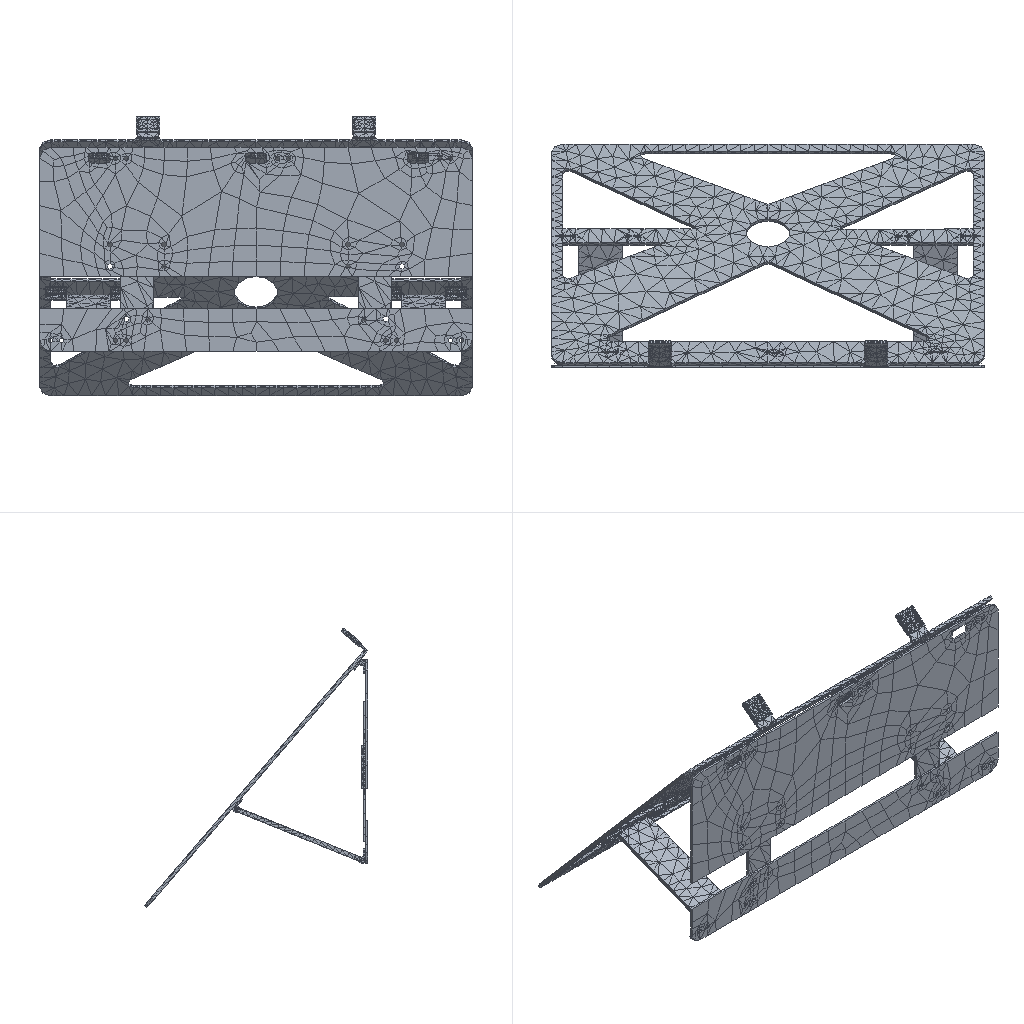Simulation study | ansys workbench
Set-up summary:
category,name,step,type,value,unit,region
solver,ansys_workbench
units,mm-N-s-tonne (MPa),,stated,"/units,MPA"
analysis,LS1,,static
load_step,LS1,LS1,static,nsubst=1; time=1
mesh,nodes,,,34982
mesh,elements,,,26385
element_type,SOLID187,,,13031
element_type,TARGE170,,,5865
element_type,CONTA174,,,5865
element_type,SURF154,,,992
element_type,SOLID186,,,632
material,Structural Steel,,E,200000,tonne s^-2 mm^-1
material,Structural Steel,,nu,0.3
material,Structural Steel,,density,7.85e-09,tonne mm^-3
material,Structural Steel,,conductivity,60.5,tonne mm s^-3 C^-1
material,Structural Steel,,specific_heat,4.34e+08,mm^2 s^-2 C^-1
material,Structural Steel,,cte,1.2e-05,C^-1
material,Structural Steel,,permeability,10000
material,Structural Steel,,resistivity,0.00017,ohm mm
load,Define Force Using Surface Effect Elements,LS1,surface-effect pres face 1,-1.28788e-17,,SURF154 #153
load,Define Force Using Surface Effect Elements,LS1,surface-effect pres face 2,-0.004879,,SURF154 #153
load,Define Force Using Surface Effect Elements,LS1,surface-effect pres face 3,-0.004202,,SURF154 #153
bc,Fixed Supports,model,fixed,[dofs=ALL],,_FIXEDSU
contact,Contact Region,,bonded (always),element=CONTA174
contact,Contact Region 2,,bonded (always),element=CONTA174
contact,Contact Region 3,,bonded (always),element=CONTA174
contact,Contact Region 4,,bonded (always),element=CONTA174
contact,Contact Region 5,,bonded (always),element=CONTA174
contact,Contact Region 6,,bonded (always),element=CONTA174
contact,Contact Region 7,,bonded (always),element=CONTA174
contact,Contact Region 8,,bonded (always),element=CONTA174
contact,Contact Region 9,,bonded (always),element=CONTA174
contact,Contact Region 10,,bonded (always),element=CONTA174
contact,Contact Region 11,,bonded (always),element=CONTA174
contact,Contact Region 12,,bonded (always),element=CONTA174
contact,Contact Region 13,,bonded (always),element=CONTA174
contact,Contact Region 14,,bonded (always),element=CONTA174
contact,Contact Region 15,,bonded (always),element=CONTA174
contact,Contact Region 16,,bonded (always),element=CONTA174
contact,Contact Region 17,,bonded (always),element=CONTA174
contact,Contact Region 18,,bonded (always),element=CONTA174
contact,Contact Region 19,,bonded (always),element=CONTA174
contact,Contact Region 20,,bonded (always),element=CONTA174
contact,Contact Region 21,,bonded (always),element=CONTA174
contact,Contact Region 22,,bonded (always),element=CONTA174
contact,Contact Region 23,,bonded (always),element=CONTA174
contact,Contact Region 24,,bonded (always),element=CONTA174
contact,Contact Region 25,,bonded (always),element=CONTA174
contact,Contact Region 26,,bonded (always),element=CONTA174
contact,Contact Region 27,,bonded (always),element=CONTA174
contact,Contact Region 28,,bonded (always),element=CONTA174
contact,Contact Region 29,,bonded (always),element=CONTA174
contact,Contact Region 30,,bonded (always),element=CONTA174
contact,Contact Region 31,,bonded (always),element=CONTA174
contact,Contact Region 32,,bonded (always),element=CONTA174
contact,Contact Region 33,,bonded (always),element=CONTA174
contact,Contact Region 34,,bonded (always),element=CONTA174
contact,Contact Region 35,,bonded (always),element=CONTA174
contact,Contact Region 36,,bonded (always),element=CONTA174
contact,Contact Region 37,,bonded (always),element=CONTA174
contact,Contact Region 38,,bonded (always),element=CONTA174
contact,Contact Region 39,,bonded (always),element=CONTA174
contact,Contact Region 40,,bonded (always),element=CONTA174
contact,Contact Region 41,,bonded (always),element=CONTA174
contact,Contact Region 42,,bonded (always),element=CONTA174
contact,Contact Region 43,,bonded (always),element=CONTA174
contact,Contact Region 44,,bonded (always),element=CONTA174
contact,Contact Region 45,,bonded (always),element=CONTA174
contact,Contact Region 46,,bonded (always),element=CONTA174
contact,Contact Region 47,,bonded (always),element=CONTA174
contact,Contact Region 48,,bonded (always),element=CONTA174
contact,Contact Region 49,,bonded (always),element=CONTA174
contact,Contact Region 50,,bonded (always),element=CONTA174
contact,Contact Region 51,,bonded (always),element=CONTA174
contact,Contact Region 52,,bonded (always),element=CONTA174
contact,Contact Region 53,,bonded (always),element=CONTA174
contact,Contact Region 54,,bonded (always),element=CONTA174
contact,Contact Region 55,,bonded (always),element=CONTA174
contact,Contact Region 56,,bonded (always),element=CONTA174
contact,Contact Region 57,,bonded (always),element=CONTA174
contact,Contact Region 58,,bonded (always),element=CONTA174
contact,Contact Region 59,,bonded (always),element=CONTA174
contact,Contact Region 60,,bonded (always),element=CONTA174
contact,Contact Region 61,,bonded (always),element=CONTA174
named_set,_FIXEDSU,,node,1923
Ansys APDL input file, long lists of numbers shortened:
/batch
/config,noeldb,1     ! force off writing results to database
*get,_wallstrt,active,,time,wall
! ANSYS input file written by Workbench version 2022 R1
! File used for geometry attach:
/title,wbnew--____ (A5)
! ****** Begin Custom Load Command Snippet ******
/COM, ACT Extensions:
/COM,     LSDYNA, 2021.1
/COM,
! ****** End   Custom Load Command Snippet ******
*DIM,_wb_ProjectScratch_dir,string,248
_wb_ProjectScratch_dir(1) = ''
*DIM,_wb_SolverFiles_dir,string,248
_wb_SolverFiles_dir(1) = ''
*DIM,_wb_userfiles_dir,string,248
_wb_userfiles_dir(1) = ''
/com,--- Data in consistent NMM units. See Solving Units in the help system for more information.
/units,MPA
/nopr
/wb,file,start              !  signify a WB generated input file
/prep7
! Turn off shape checking because checks already performed inside WB mesher.
! See help system for more information.
SHPP,OFF,,NOWARN
/nolist
etcon,set             ! allow ANSYS to choose best KEYOP's for 180x elements, resets any applicable keyopt to MAPDL defaults
/com,*********** Nodes for the whole assembly ***********
nblock,3,,38480
(1i9,3e20.9e3)
        1     3.182810886E+02     2.161891006E+02     1.535110388E+02
! (34981 more lines like these left out)
-1
/wb,elem,start            !  set before creation of elements
/com,*********** Elements for Body 1 "fromt_backplate_with_mount_assy___ _________|front-backplate___ _________|__________2" ***********
et,1,186
keyo,1,2,1          ! set full integration on SOLID186
eblock,19,solid,,359
(19i9)
        1        1        1        1        0        0        0        0       20        0    13305    32083    32585    32584    32687    32522    32888    32889    32789
! (717 more lines like these left out)
-1
/com,*********** Elements for Body 2 "fromt_backplate_with_mount_assy___ _________|sliding_system_mount___ _________|_______-________2" ***********
et,2,187
eblock,19,solid,,223
(19i9)
        2        2        2        2        0        0        0        0       10        0     1339     3144     3192     3145     3200     3429     3434     3426     3430
! (445 more lines like these left out)
-1
/com,*********** Elements for Body 3 "fromt_backplate_with_mount_assy___ _________|sliding_system_mount___ _________|_______-________2[2]" ***********
et,3,187
eblock,19,solid,,223
(19i9)
        3        3        3        3        0        0        0        0       10        0    11173    26097    26145    26098    26153    26382    26387    26379    26383
! (445 more lines like these left out)
-1
/com,*********** Elements for Body 4 "fromt_backplate_with_mount_assy___ _________|sliding_system_mount___ _________|_______-________2[3]" ***********
et,4,187
eblock,19,solid,,223
(19i9)
        4        4        4        4        0        0        0        0       10        0     1562     3692     3740     3693     3748     3977     3982     3974     3978
! (445 more lines like these left out)
-1
/com,*********** Elements for Body 5 "fromt_backplate_with_mount_assy___ _________|sliding_system_mount___ _________|_______-________2[4]" ***********
et,5,187
eblock,19,solid,,223
(19i9)
        5        5        5        5        0        0        0        0       10        0     2179     5406     5454     5407     5462     5691     5696     5688     5692
! (445 more lines like these left out)
-1
! (25 more sections like these left out)
/wb,elem,end               !  done creating elements
/com,*********** Send User Defined Coordinate System(s) ***********
csys,0
toffst,273.15,  ! Temperature offset from absolute zero
/com,*********** Set Reference Temperature ***********
tref,22.
/wb,mat,start              !  starting to send materials
/com,*********** Send Materials ***********
Temperature = 'TEMP' ! Temperature
MP,DENS,1,7.85e-09,	! tonne mm^-3
MP,ALPX,1,1.2e-05,	! C^-1
MP,C,1,434000000,	! mm^2 s^-2 C^-1
MP,KXX,1,60.5,	! tonne mm s^-3 C^-1
MP,RSVX,1,0.00017,	! ohm mm
MP,EX,1,200000,	! tonne s^-2 mm^-1
MP,NUXY,1,0.3,
MP,MURX,1,10000,
Temperature = 'TEMP' ! Temperature
MP,DENS,2,7.85e-09,	! tonne mm^-3
MP,ALPX,2,1.2e-05,	! C^-1
MP,C,2,434000000,	! mm^2 s^-2 C^-1
MP,KXX,2,60.5,	! tonne mm s^-3 C^-1
MP,RSVX,2,0.00017,	! ohm mm
MP,EX,2,200000,	! tonne s^-2 mm^-1
MP,NUXY,2,0.3,
MP,MURX,2,10000,
Temperature = 'TEMP' ! Temperature
MP,DENS,3,7.85e-09,	! tonne mm^-3
MP,ALPX,3,1.2e-05,	! C^-1
MP,C,3,434000000,	! mm^2 s^-2 C^-1
MP,KXX,3,60.5,	! tonne mm s^-3 C^-1
MP,RSVX,3,0.00017,	! ohm mm
MP,EX,3,200000,	! tonne s^-2 mm^-1
MP,NUXY,3,0.3,
MP,MURX,3,10000,
Temperature = 'TEMP' ! Temperature
MP,DENS,4,7.85e-09,	! tonne mm^-3
MP,ALPX,4,1.2e-05,	! C^-1
MP,C,4,434000000,	! mm^2 s^-2 C^-1
MP,KXX,4,60.5,	! tonne mm s^-3 C^-1
MP,RSVX,4,0.00017,	! ohm mm
MP,EX,4,200000,	! tonne s^-2 mm^-1
MP,NUXY,4,0.3,
MP,MURX,4,10000,
Temperature = 'TEMP' ! Temperature
MP,DENS,5,7.85e-09,	! tonne mm^-3
MP,ALPX,5,1.2e-05,	! C^-1
MP,C,5,434000000,	! mm^2 s^-2 C^-1
MP,KXX,5,60.5,	! tonne mm s^-3 C^-1
MP,RSVX,5,0.00017,	! ohm mm
MP,EX,5,200000,	! tonne s^-2 mm^-1
MP,NUXY,5,0.3,
MP,MURX,5,10000,
Temperature = 'TEMP' ! Temperature
MP,DENS,6,7.85e-09,	! tonne mm^-3
MP,ALPX,6,1.2e-05,	! C^-1
MP,C,6,434000000,	! mm^2 s^-2 C^-1
MP,KXX,6,60.5,	! tonne mm s^-3 C^-1
MP,RSVX,6,0.00017,	! ohm mm
MP,EX,6,200000,	! tonne s^-2 mm^-1
MP,NUXY,6,0.3,
MP,MURX,6,10000,
Temperature = 'TEMP' ! Temperature
MP,DENS,7,7.85e-09,	! tonne mm^-3
MP,ALPX,7,1.2e-05,	! C^-1
MP,C,7,434000000,	! mm^2 s^-2 C^-1
MP,KXX,7,60.5,	! tonne mm s^-3 C^-1
MP,RSVX,7,0.00017,	! ohm mm
MP,EX,7,200000,	! tonne s^-2 mm^-1
MP,NUXY,7,0.3,
MP,MURX,7,10000,
Temperature = 'TEMP' ! Temperature
MP,DENS,8,7.85e-09,	! tonne mm^-3
MP,ALPX,8,1.2e-05,	! C^-1
MP,C,8,434000000,	! mm^2 s^-2 C^-1
MP,KXX,8,60.5,	! tonne mm s^-3 C^-1
MP,RSVX,8,0.00017,	! ohm mm
MP,EX,8,200000,	! tonne s^-2 mm^-1
MP,NUXY,8,0.3,
MP,MURX,8,10000,
Temperature = 'TEMP' ! Temperature
MP,DENS,9,7.85e-09,	! tonne mm^-3
MP,ALPX,9,1.2e-05,	! C^-1
MP,C,9,434000000,	! mm^2 s^-2 C^-1
MP,KXX,9,60.5,	! tonne mm s^-3 C^-1
MP,RSVX,9,0.00017,	! ohm mm
MP,EX,9,200000,	! tonne s^-2 mm^-1
! (191 more lines like these left out)
/wb,mat,end                !  done sending materials
!************************* Model Summary ********************
!fromt_backplate_with_mount_assy___ _________|front-backplate___ _________|__________2,	结构钢,	matid,	1
!fromt_backplate_with_mount_assy___ _________|sliding_system_mount___ _________|_______-________2,	结构钢,	matid,	2
!fromt_backplate_with_mount_assy___ _________|sliding_system_mount___ _________|_______-________2[2],	结构钢,	matid,	3
! (29 more lines like these left out)
*get,_xmin,node,,mnloc,x
*get,_ymin,node,,mnloc,y
*get,_zmin,node,,mnloc,z
*get,_xmax,node,,mxloc,x
*get,_ymax,node,,mxloc,y
*get,_zmax,node,,mxloc,z
_ASMDIAG=(_xmax-_xmin)*(_xmax-_xmin)+(_ymax-_ymin)*(_ymax-_ymin)+(_zmax-_zmin)*(_zmax-_zmin)
_ASMDIAG=SQRT(_ASMDIAG)
/wb,contact,start          !  starting to send contact
/com,*********** Create Contact "接触区域" ***********
/com,            Real Constant Set For Above Contact Is 32 & 31
*set,tid,32
*set,cid,31
r,tid
r,cid
et,tid,170
et,cid,174
eblock,10,,,30
(15i9)
    26408       32       32       32        0    32628    32629    32088    32302    34569    33086    33083    33780
! (29 more lines like these left out)
-1
eblock,10,,,30
(15i9)
    26438       31       31       31        0    32628    32629    32088    32302    34569    33086    33083    33780
! (29 more lines like these left out)
-1
eblock,10,,,40
(15i9)
    26468       31       32       31        0     3152     3157     3158     3158     3459     3480     3158     3460
! (39 more lines like these left out)
-1
eblock,10,,,40
(15i9)
    26508       32       31       32        0     3152     3157     3158     3158     3459     3480     3158     3460
! (39 more lines like these left out)
-1
keyo,cid,8,2               ! auto create asymmetric contact (from Program Controlled setting)
keyo,cid,10,0              ! adjust contact stiffness each NR iteration (from Program Controlled setting)
keyo,cid,12,5              ! bonded always
keyo,cid,18,1              ! small sliding turned on by application
keyo,cid,2,0               ! augmented Lagrange (from Program Controlled setting)
keyo,cid,4,0               ! on Gauss point (from Program Controlled setting)
keyo,cid,9,1               ! ignore initial gaps/penetration
keyo,cid,7,0               ! No Prediction
rmod,tid,3,10.      ! FKN
rmod,tid,5,0.       ! ICONT
rmod,tid,6,0.       ! PINB
rmod,tid,10,0.      ! CNOF
rmod,tid,12,0.      ! FKT
rmod,tid,36,113     ! WB DSID
rmod,cid,3,10.      ! FKN
rmod,cid,5,0.       ! ICONT
rmod,cid,6,0.       ! PINB
rmod,cid,10,0.      ! CNOF
rmod,cid,12,0.      ! FKT
rmod,cid,36,113     ! WB DSID
/com,*********** Create Contact "接触区域 2" ***********
/com,            Real Constant Set For Above Contact Is 34 & 33
*set,tid,34
*set,cid,33
r,tid
r,cid
et,tid,170
et,cid,174
eblock,10,,,30
(15i9)
    26548       34       34       34        0    32142    32258    32259    32293    33301    33692    33696    33302
! (29 more lines like these left out)
-1
eblock,10,,,30
(15i9)
    26578       33       33       33        0    32142    32258    32259    32293    33301    33692    33696    33302
! (29 more lines like these left out)
-1
eblock,10,,,40
(15i9)
    26608       33       34       33        0    26105    26110    26111    26111    26412    26433    26111    26413
! (39 more lines like these left out)
-1
eblock,10,,,40
(15i9)
    26648       34       33       34        0    26105    26110    26111    26111    26412    26433    26111    26413
! (39 more lines like these left out)
-1
keyo,cid,8,2               ! auto create asymmetric contact (from Program Controlled setting)
keyo,cid,10,0              ! adjust contact stiffness each NR iteration (from Program Controlled setting)
keyo,cid,12,5              ! bonded always
keyo,cid,18,1              ! small sliding turned on by application
keyo,cid,2,0               ! augmented Lagrange (from Program Controlled setting)
keyo,cid,4,0               ! on Gauss point (from Program Controlled setting)
keyo,cid,9,1               ! ignore initial gaps/penetration
keyo,cid,7,0               ! No Prediction
rmod,tid,3,10.      ! FKN
rmod,tid,5,0.       ! ICONT
rmod,tid,6,0.       ! PINB
rmod,tid,10,0.      ! CNOF
rmod,tid,12,0.      ! FKT
rmod,tid,36,116     ! WB DSID
rmod,cid,3,10.      ! FKN
rmod,cid,5,0.       ! ICONT
rmod,cid,6,0.       ! PINB
rmod,cid,10,0.      ! CNOF
rmod,cid,12,0.      ! FKT
rmod,cid,36,116     ! WB DSID
/com,*********** Create Contact "接触区域 3" ***********
/com,            Real Constant Set For Above Contact Is 36 & 35
*set,tid,36
*set,cid,35
r,tid
r,cid
et,tid,170
et,cid,174
eblock,10,,,28
(15i9)
    26688       36       36       36        0    32119    32092    32138    32091    33104    33105    33098    33097
! (27 more lines like these left out)
-1
eblock,10,,,28
(15i9)
    26716       35       35       35        0    32119    32092    32138    32091    33104    33105    33098    33097
! (27 more lines like these left out)
-1
eblock,10,,,40
(15i9)
    26744       35       36       35        0     3700     3705     3706     3706     4007     4028     3706     4008
! (39 more lines like these left out)
-1
eblock,10,,,40
(15i9)
    26784       36       35       36        0     3700     3705     3706     3706     4007     4028     3706     4008
! (39 more lines like these left out)
-1
keyo,cid,8,2               ! auto create asymmetric contact (from Program Controlled setting)
keyo,cid,10,0              ! adjust contact stiffness each NR iteration (from Program Controlled setting)
keyo,cid,12,5              ! bonded always
keyo,cid,18,1              ! small sliding turned on by application
keyo,cid,2,0               ! augmented Lagrange (from Program Controlled setting)
keyo,cid,4,0               ! on Gauss point (from Program Controlled setting)
keyo,cid,9,1               ! ignore initial gaps/penetration
keyo,cid,7,0               ! No Prediction
rmod,tid,3,10.      ! FKN
rmod,tid,5,0.       ! ICONT
rmod,tid,6,0.       ! PINB
rmod,tid,10,0.      ! CNOF
rmod,tid,12,0.      ! FKT
rmod,tid,36,119     ! WB DSID
rmod,cid,3,10.      ! FKN
rmod,cid,5,0.       ! ICONT
rmod,cid,6,0.       ! PINB
rmod,cid,10,0.      ! CNOF
rmod,cid,12,0.      ! FKT
rmod,cid,36,119     ! WB DSID
/com,*********** Create Contact "接触区域 4" ***********
/com,            Real Constant Set For Above Contact Is 38 & 37
*set,tid,38
*set,cid,37
r,tid
r,cid
et,tid,170
et,cid,174
eblock,10,,,29
(15i9)
    26824       38       38       38        0    32119    32092    32138    32091    33104    33105    33098    33097
! (28 more lines like these left out)
-1
eblock,10,,,29
(15i9)
    26853       37       37       37        0    32119    32092    32138    32091    33104    33105    33098    33097
! (28 more lines like these left out)
-1
eblock,10,,,40
(15i9)
    26882       37       38       37        0     5414     5419     5420     5420     5721     5742     5420     5722
! (39 more lines like these left out)
-1
eblock,10,,,40
(15i9)
    26922       38       37       38        0     5414     5419     5420     5420     5721     5742     5420     5722
! (39 more lines like these left out)
-1
keyo,cid,8,2               ! auto create asymmetric contact (from Program Controlled setting)
keyo,cid,10,0              ! adjust contact stiffness each NR iteration (from Program Controlled setting)
keyo,cid,12,5              ! bonded always
keyo,cid,18,1              ! small sliding turned on by application
keyo,cid,2,0               ! augmented Lagrange (from Program Controlled setting)
keyo,cid,4,0               ! on Gauss point (from Program Controlled setting)
keyo,cid,9,1               ! ignore initial gaps/penetration
keyo,cid,7,0               ! No Prediction
rmod,tid,3,10.      ! FKN
rmod,tid,5,0.       ! ICONT
rmod,tid,6,0.       ! PINB
rmod,tid,10,0.      ! CNOF
rmod,tid,12,0.      ! FKT
rmod,tid,36,122     ! WB DSID
rmod,cid,3,10.      ! FKN
rmod,cid,5,0.       ! ICONT
rmod,cid,6,0.       ! PINB
rmod,cid,10,0.      ! CNOF
rmod,cid,12,0.      ! FKT
rmod,cid,36,122     ! WB DSID
/com,*********** Create Contact "接触区域 5" ***********
/com,            Real Constant Set For Above Contact Is 40 & 39
*set,tid,40
*set,cid,39
r,tid
r,cid
et,tid,170
et,cid,174
eblock,10,,,25
(15i9)
    26962       40       40       40        0    32628    32629    32088    32302    34569    33086    33083    33780
! (24 more lines like these left out)
-1
eblock,10,,,25
(15i9)
    26987       39       39       39        0    32628    32629    32088    32302    34569    33086    33083    33780
! (24 more lines like these left out)
-1
eblock,10,,,15
(15i9)
    27012       39       40       39        0     5087     5079     5006     5009     5341     5194     5191     5203
! (14 more lines like these left out)
-1
eblock,10,,,15
(15i9)
    27027       40       39       40        0     5087     5079     5006     5009     5341     5194     5191     5203
! (14 more lines like these left out)
-1
keyo,cid,8,2               ! auto create asymmetric contact (from Program Controlled setting)
keyo,cid,10,0              ! adjust contact stiffness each NR iteration (from Program Controlled setting)
keyo,cid,12,5              ! bonded always
keyo,cid,18,1              ! small sliding turned on by application
keyo,cid,2,0               ! augmented Lagrange (from Program Controlled setting)
keyo,cid,4,0               ! on Gauss point (from Program Controlled setting)
keyo,cid,9,1               ! ignore initial gaps/penetration
keyo,cid,7,0               ! No Prediction
rmod,tid,3,10.      ! FKN
rmod,tid,5,0.       ! ICONT
rmod,tid,6,0.       ! PINB
rmod,tid,10,0.      ! CNOF
rmod,tid,12,0.      ! FKT
rmod,tid,36,125     ! WB DSID
rmod,cid,3,10.      ! FKN
rmod,cid,5,0.       ! ICONT
rmod,cid,6,0.       ! PINB
rmod,cid,10,0.      ! CNOF
rmod,cid,12,0.      ! FKT
rmod,cid,36,125     ! WB DSID
! (56 more sections like these left out)
/wb,contact,end            !  done creating contacts
/golist
/wb,load,start             !  starting to send loads
/com,*********** Fixed Supports ***********
CMBLOCK,_FIXEDSU,NODE,     1923
(8i10)
     30176     30177     30178     30179     30180     30181     30182     30183
! (240 more lines like these left out)
cmsel,s,_FIXEDSU
d,all,all
nsel,all
/com,*********** Define Force Using Surface Effect Elements ***********
local,12,0,0.,0.,0.,0.,0.,0.
csys,0
et,153,154
eblock,10,,,992
(15i9)
    38138      153      153      153       12    11615    12008    11616    11616    14263    14269    11616    14260
! (991 more lines like these left out)
-1
esel,s,type,,153
keyop,153,2,1                ! Apply load in local coordinate system
keyop,153,7,1                ! Use original area so load is constant in large deformation
esel,all
/gst,on,on
fini
*get,_numnode,node,0,count
*get,_numelem,elem,0,count
*get, _MAXELEMNUM, elem, 0, NUM, MAX
*get, _MAXNODENUM, node, 0, NUM, MAX
*get, _MAXELEMTYPE, etyp, 0, NUM, MAX
*get, _MAXREALCONST, real, 0, NUM, MAX
/go
/wb,load,end               !  done creating loads
/com,--- Number of total nodes = %_numnode%
/com,--- Number of contact elements = 12722
/com,--- Number of spring elements = 0
/com,--- Number of bearing elements = 0
/com,--- Number of solid elements = 13663
/com,--- Number of condensed parts = 0
/com,--- Number of total elements = %_numelem%
*get,_wallbsol,active,,time,wall
/com,****************************************************************************
/com,*************************    SOLUTION       ********************************
/com,****************************************************************************
/solu
antype,0                   ! static analysis
_thickRatio=  0     ! Ratio of thick parts in the model
eqsl,sparse,,,,,1
cntr,print,1               ! print out contact info and also make no initial contact an error
dmpoption,emat,no             ! Don't combine emat file for DANSYS
dmpoption,esav,no             ! Don't combine esav file for DANSYS
nldiag,cont,iter           ! print out contact info each equilibrium iteration
rescontrol,,none                 ! Do not keep any restart files
/com,****************************************************
/com,******************* SOLVE FOR LS 1 OF 1 ****************
esel,s,type,,153
nsle
sfe,all,1,pres,1,-1.28787677236801e-017
sfe,all,2,pres,1,-4.87918117754962e-003
sfe,all,3,pres,1,-4.20229193473377e-003
nsel,all
esel,all
/nopr
/gopr
nsub,1,1,1
time,1.
outres,erase
outres,all,none
outres,nsol,all,
outres,rsol,all
outres,eangl,all
outres,etmp,all
outres,veng,all
outres,strs,all,
outres,epel,all,
outres,eppl,all,
outres,cont,all,
! *********** WB SOLVE COMMAND ***********
! check interactive state
*get,ANSINTER_,active,,int
*if,ANSINTER_,ne,0,then
/eof
*endif
solve
/com *************** Write FE CONNECTORS *********
CEWRITE,file,ce,,INTE
/com,****************************************************
/com,*************** FINISHED SOLVE FOR LS 1 *************
*get,_wallasol,active,,time,wall
/nopr
*get,_numnode,node,0,count
*get,_numelem,elem,0,count
*get, _MAXELEMNUM, elem, 0, NUM, MAX
*get, _MAXNODENUM, node, 0, NUM, MAX,,,INTERNAL
*get, _MAXELEMTYPE, etyp, 0, NUM, MAX
*get, _MAXREALCONST, real, 0, NUM, MAX
/gopr
/post1
xmlo,ENCODING,ISO-8859-1
xmlo,parm
/xml,parm,xml
fini
/gopr
*get,_walldone,active,,time,wall
_preptime=(_wallbsol-_wallstrt)*3600
_solvtime=(_wallasol-_wallbsol)*3600
_posttime=(_walldone-_wallasol)*3600
_totaltim=(_walldone-_wallstrt)*3600
*get,_dlbratio,active,0,solu,dlbr
*get,_combtime,active,0,solu,comb
*get,_ssmode,active,0,solu,ssmm
*get,_ndofs,active,0,solu,ndof
*get,_sol_end_time,active,0,set,time
*if,_sol_end_time,eq,1.,then
/fclean				!clean distributed files
*endif
/com,--- Total number of nodes = %_numnode%
/com,--- Total number of elements = %_numelem%
/com,--- Element load balance ratio = %_dlbratio%
/com,--- Time to combine distributed files = %_combtime%
/com,--- Sparse memory mode = %_ssmode%
/com,--- Number of DOF = %_ndofs%
/wb,file,end               ! done with WB generated input
Results summary:
result,analyses[0].index,,,1
result,analyses[0].system,,,SYS
result,analyses[0].deck,,,deck.dat
result,analyses[0].solve_status,,,completed
result,analyses[0].analysis_type,,,static
result,analyses[0].physics,,,mechanical
result,analyses[0].unit_system,,,"NMM: mm, ton, N, s, mV, mA, degC"
result,analyses[0].n_sets,,,1
result,analyses[0].load_steps[0].set,set=1,,1
result,analyses[0].load_steps[0].time_or_freq,set=1,,1
result,analyses[0].load_steps[0].max_displacement_magnitude,set=1,,1.974
result,analyses[0].load_steps[0].max_von_mises_nodal,set=1,,246.95
result,analyses[0].load_steps[0].reaction_force_sum_xyz[1],set=1,,-7.96984e-07
result,analyses[0].load_steps[0].reaction_force_sum_xyz[2],set=1,,378.855
result,analyses[0].load_steps[0].reaction_force_sum_xyz[3],set=1,,326.296